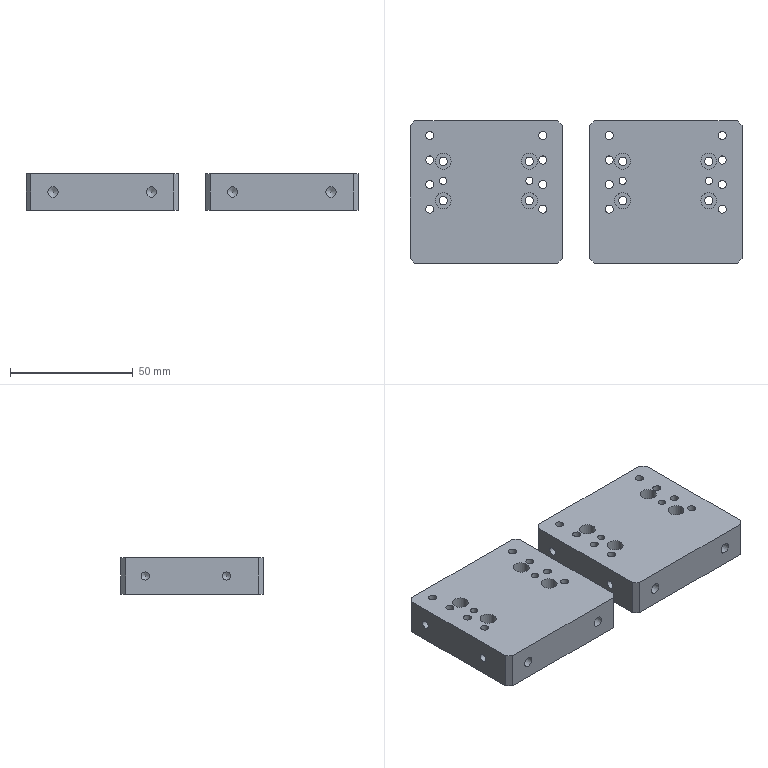CAM job | NX | 3-axis milling, drilling | part box 135 x 58 x 15 mm | stock box 140 x 63 x 20 mm
Tools:
number,name,description,diameter,corner_radius,flute_length,length,flutes
4,D4,平底铣刀-粗,4.0,0.0,25.0,75.0,2
9,D10,平底铣刀-粗,10.0,0.0,35.0,75.0,2
11,D4-J,平底铣刀-精,4.0,0.0,50.0,75.0,2
7,D6-J,平底铣刀-精,6.0,0.0,25.0,75.0,2
1,D80R0.8飞刀,圆鼻刀-粗,80.0,0.8,50.0,75.0,2
1,D80R0.8飞刀-J,圆鼻刀-精,80.0,0.8,50.0,75.0,2
2,D6倒角刀,倒角刀,6.0,0.0,3.0,25.0,2
21,M4X0.7,丝锥,3.3,0.0,35.0,50.0,2
18,D3铰刀,Drilling Tool,3.0,0.0,75.0,100.0,6
13,ZT3.4,钻头,3.4,0.0,35.0,50.0,2
17,ZT2.9,Drilling Tool,2.9,0.0,35.0,50.0,2
Operations:
program,operation,operation_type,tool,method,geometry_group,spindle_rpm,surface_speed,feed_per_tooth,feed_cut,feed_plunge,cut_length_mm,path_length_mm,cut_time_min,machine_time_min
B,FLOORWALL_FACEONECUTROUGH_COPY,VolumeBased25DMillingOperation,D80R0.8飞刀,ZLEVELROUGH-DEPTHK-STEPG,W-B,2800.0,703.696,0.5357,3000.0,100.0,2188.746,4660.966,0.7296,0.9768
B,FLOORWALL_FACEONECUTFINISH_COPY,VolumeBased25DMillingOperation,D80R0.8飞刀-J,SIDEFINISH-DEPTHK-STEPG,W-B,4000.0,1005.28,0.125,1000.0,100.0,242.998,338.998,0.243,0.2526
B,NG_DRILLCHAMFER_3,Operation,D6倒角刀,METHOD,W-B,8000.0,150.796,0.0625,1000.0,0.0,19.2,255.775,0.0192,0.0429
B,NG_DRILLCHAMFER_4,Operation,D6倒角刀,METHOD,W-B,8000.0,150.796,0.0625,1000.0,0.0,40.0,374.49,0.04,0.0734
B,NG_DRILLCHAMFER_5,Operation,D6倒角刀,METHOD,W-B,8000.0,150.796,0.0625,1000.0,0.0,83.2,556.045,0.0832,0.1305
B,C0.3_CLOSEDCONTOURCHAMFER6X45L_COPY,PlanarMilling,D6倒角刀,CLIMBFACE_CHAMFER-DEPTH0-STEPG,W-B,7000.0,131.0,0.1071,1500.0,100.0,252.842,348.842,0.1686,0.1782
B,C0.3_CLOSEDCONTOURCHAMFER6X45L_COPY_1,PlanarMilling,D6倒角刀,CLIMBFACE_CHAMFER-DEPTH0-STEPG,W-B,7000.0,131.0,0.1071,1500.0,100.0,252.842,348.842,0.1686,0.1782
A,TOPFACE,FaceMilling,D80R0.8飞刀,SIDEFINISH-DEPTHK-STEPG,W-A,4500.0,1385.0,0.1667,1500.0,100.0,229.0,325.0,0.1527,0.1623
A,PROFILE_ROUGH_2,VolumeBased25DMillingOperation,D10,METHOD,W-A,8000.0,251.327,0.375,6000.0,80.0,11232.079,11532.579,1.872,1.902
A,SPOTDRILL-DEPTH0.8,Operation,D6倒角刀,NONE,W-A,8000.0,150.796,0.0312,500.0,90.0,50.4,509.478,0.1008,0.1467
A,THRUHOLE-PRECISION3.0_PILOT,Operation,ZT2.9,NONE,W-A,3200.0,29.154,0.0312,200.0,90.0,79.349,369.739,0.3967,0.4258
A,THRUHOLE-M4TAPDRILL,Operation,ZT3.4,NONE,W-A,3000.0,31.102,0.05,300.0,90.0,352.0,1058.639,1.173,1.244
A,COUNTERBORE-DRILL_SEG0,Operation,ZT3.4,NONE,W-A,2800.0,29.908,0.0179,100.0,90.0,152.172,583.51,1.522,1.565
A,HOLEROUGHD4_1,CylinderMilling,D4,NONE,W-A,8000.0,100.531,0.075,1200.0,100.0,2111.637,3178.637,1.76,1.866
A,HOLEFINISHD4_1,CylinderMilling,D4-J,FINISHSTEPDEPTHOFF,W-A,8000.0,100.531,0.0312,500.0,100.0,249.968,1316.968,0.4999,0.6066
A,SELBODYONLY,SurfaceContour,D6倒角刀,METHOD,W-A,8000.0,150.796,0.1875,3000.0,100.0,505.231,747.461,0.1684,0.1926
A,NG_DRILLCHAMFER_1,Operation,D6倒角刀,METHOD,W-A,8000.0,150.796,0.0312,500.0,0.0,19.2,255.775,0.0384,0.0621
A,NG_DRILLCHAMFER_2,Operation,D6倒角刀,METHOD,W-A,8000.0,150.796,0.0312,500.0,0.0,83.2,556.045,0.1664,0.2137
A,MILLCHAMFER_1,PlanarMilling,D6倒角刀,NONE,W-A,8000.0,150.796,0.0312,500.0,100.0,234.043,1162.961,0.4681,0.561
A,THRUHOLE-TAPM4,Operation,M4X0.7,METHOD,W-A,600.0,6.22,0.0006,0.7,90.0,304.0,962.639,434.286,434.352
A,REAMING,Operation,D3铰刀,METHOD,W-A,500.0,4.712,0.0167,50.0,0.0,68.0,347.042,1.36,1.388
A,PROFILE_SEMIFINISH_2,VolumeBased25DMillingOperation,D6-J,METHOD,W-A,9000.0,169.646,0.0667,1200.0,100.0,1036.318,1602.876,0.8636,0.9203